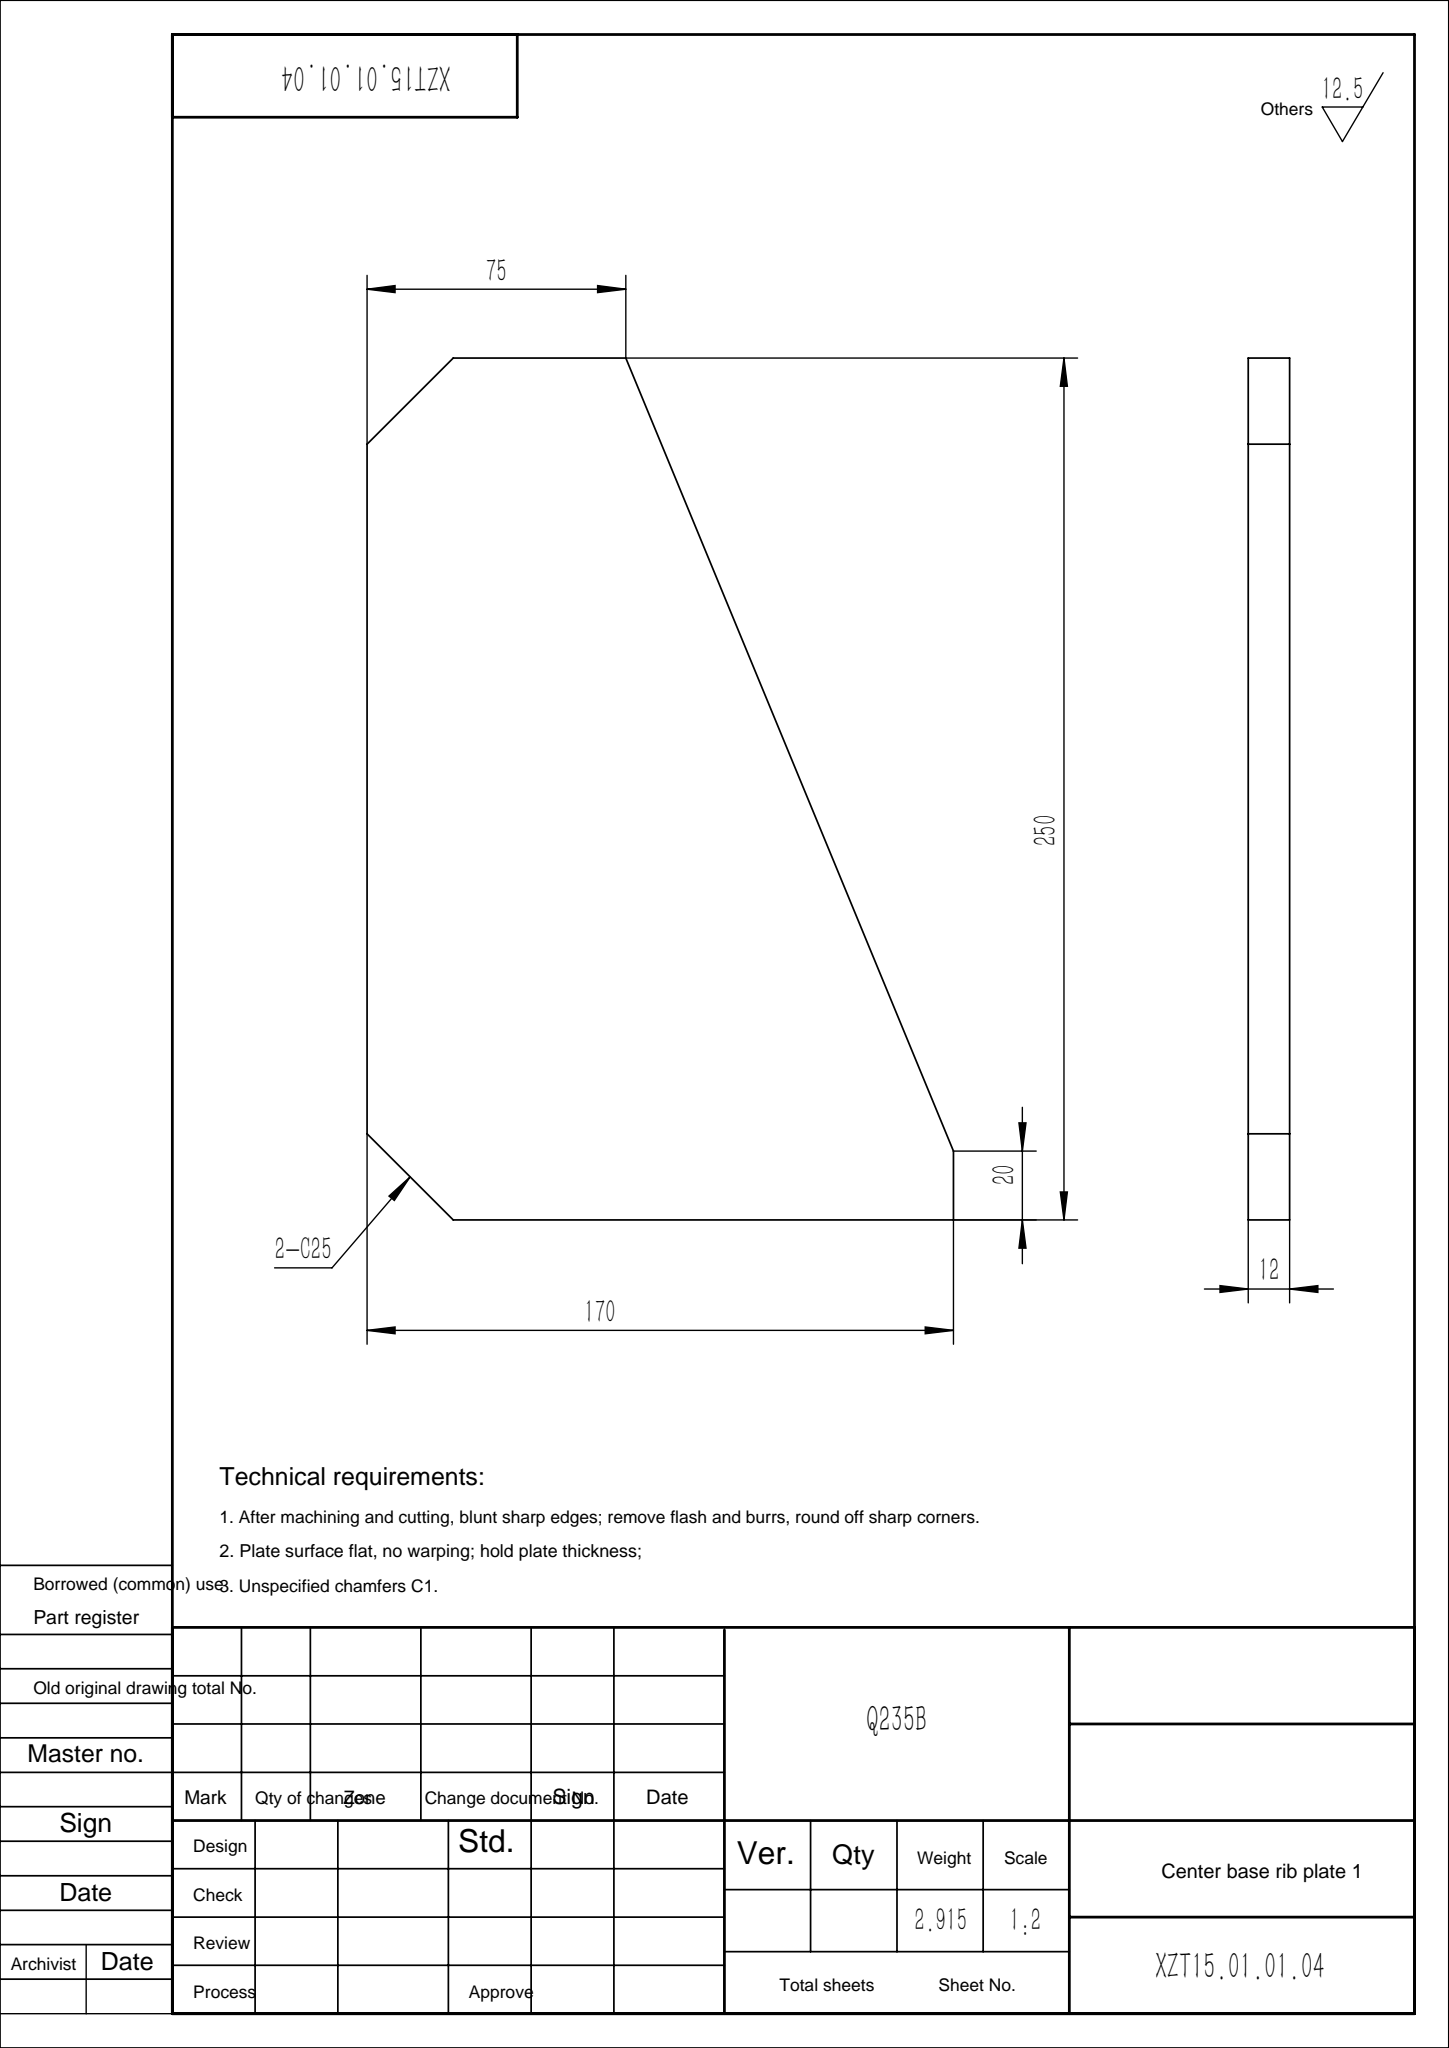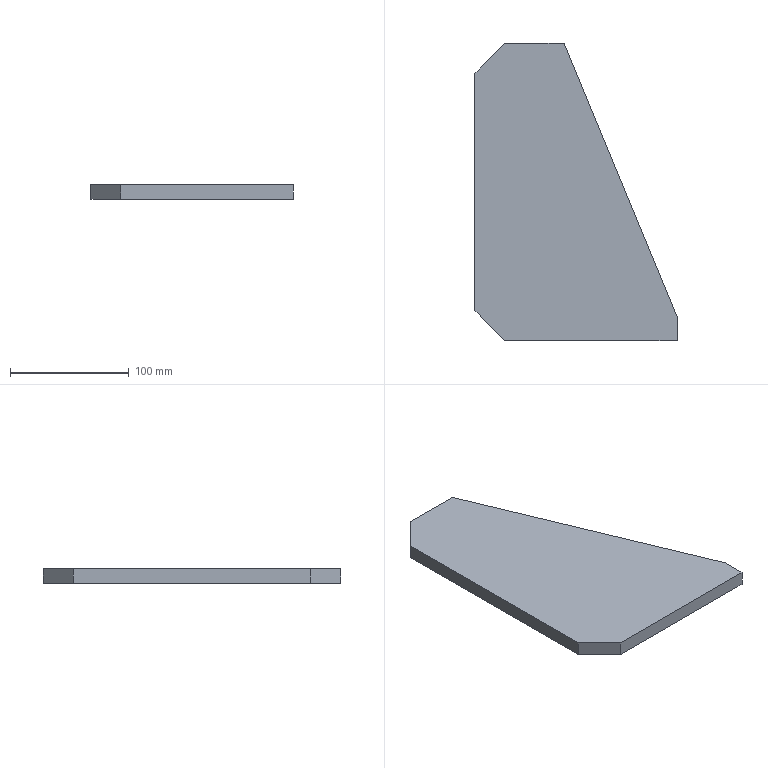Part | SolidWorks | features Chamfer 1, Extrusion 1 | 1 solid | 9 faces | box 170 x 250 x 12 mm | volume 371400 mm3 | plane 9
STEP:
#1=CARTESIAN_POINT('',(0.,225.,6.));
#2=VERTEX_POINT('',#1);
#3=CARTESIAN_POINT('',(0.,25.,6.));
#4=VERTEX_POINT('',#3);
#5=CARTESIAN_POINT('',(0.,250.,6.));
#6=DIRECTION('',(0.,-1.,0.));
#7=VECTOR('',#6,1000.);
#8=LINE('',#5,#7);
#9=EDGE_CURVE('',#2,#4,#8,.T.);
#10=ORIENTED_EDGE('',*,*,#9,.F.);
#11=CARTESIAN_POINT('',(0.,225.,-6.));
#12=VERTEX_POINT('',#11);
#13=CARTESIAN_POINT('',(0.,225.,6.));
#14=DIRECTION('',(0.,0.,-1.));
#15=VECTOR('',#14,1000.);
#16=LINE('',#13,#15);
#17=EDGE_CURVE('',#2,#12,#16,.T.);
#18=ORIENTED_EDGE('',*,*,#17,.T.);
#19=CARTESIAN_POINT('',(0.,25.,-6.));
#20=VERTEX_POINT('',#19);
#21=CARTESIAN_POINT('',(0.,250.,-6.));
#22=DIRECTION('',(0.,-1.,0.));
#23=VECTOR('',#22,1000.);
#24=LINE('',#21,#23);
#25=EDGE_CURVE('',#12,#20,#24,.T.);
#26=ORIENTED_EDGE('',*,*,#25,.T.);
#27=CARTESIAN_POINT('',(0.,25.,6.));
#28=DIRECTION('',(0.,0.,1.));
#29=VECTOR('',#28,1000.);
#30=LINE('',#27,#29);
#31=EDGE_CURVE('',#20,#4,#30,.T.);
#32=ORIENTED_EDGE('',*,*,#31,.T.);
#33=EDGE_LOOP('',(#10,#18,#26,#32));
#34=FACE_OUTER_BOUND('',#33,.T.);
#35=CARTESIAN_POINT('',(0.,250.,6.));
#36=DIRECTION('',(1.,0.,0.));
#37=DIRECTION('',(0.,1.,0.));
#38=AXIS2_PLACEMENT_3D('',#35,#36,#37);
#39=PLANE('',#38);
#40=ADVANCED_FACE('',(#34),#39,.F.);
#41=CARTESIAN_POINT('',(25.,0.,6.));
#42=VERTEX_POINT('',#41);
#43=CARTESIAN_POINT('',(170.,0.,6.));
#44=VERTEX_POINT('',#43);
#45=CARTESIAN_POINT('',(0.,0.,6.));
#46=DIRECTION('',(1.,0.,0.));
#47=VECTOR('',#46,1000.);
#48=LINE('',#45,#47);
#49=EDGE_CURVE('',#42,#44,#48,.T.);
#50=ORIENTED_EDGE('',*,*,#49,.F.);
#51=CARTESIAN_POINT('',(25.,0.,-6.));
#52=VERTEX_POINT('',#51);
#53=CARTESIAN_POINT('',(25.,0.,6.));
#54=DIRECTION('',(0.,0.,-1.));
#55=VECTOR('',#54,1000.);
#56=LINE('',#53,#55);
#57=EDGE_CURVE('',#42,#52,#56,.T.);
#58=ORIENTED_EDGE('',*,*,#57,.T.);
#59=CARTESIAN_POINT('',(170.,0.,-6.));
#60=VERTEX_POINT('',#59);
#61=CARTESIAN_POINT('',(0.,0.,-6.));
#62=DIRECTION('',(1.,0.,0.));
#63=VECTOR('',#62,1000.);
#64=LINE('',#61,#63);
#65=EDGE_CURVE('',#52,#60,#64,.T.);
#66=ORIENTED_EDGE('',*,*,#65,.T.);
#67=CARTESIAN_POINT('',(170.,0.,6.));
#68=DIRECTION('',(0.,0.,-1.));
#69=VECTOR('',#68,1000.);
#70=LINE('',#67,#69);
#71=EDGE_CURVE('',#44,#60,#70,.T.);
#72=ORIENTED_EDGE('',*,*,#71,.F.);
#73=EDGE_LOOP('',(#50,#58,#66,#72));
#74=FACE_OUTER_BOUND('',#73,.T.);
#75=CARTESIAN_POINT('',(0.,0.,6.));
#76=DIRECTION('',(0.,1.,0.));
#77=DIRECTION('',(0.,0.,1.));
#78=AXIS2_PLACEMENT_3D('',#75,#76,#77);
#79=PLANE('',#78);
#80=ADVANCED_FACE('',(#74),#79,.F.);
#81=CARTESIAN_POINT('',(170.,20.,-6.));
#82=VERTEX_POINT('',#81);
#83=CARTESIAN_POINT('',(170.,0.,-6.));
#84=DIRECTION('',(0.,1.,0.));
#85=VECTOR('',#84,1000.);
#86=LINE('',#83,#85);
#87=EDGE_CURVE('',#60,#82,#86,.T.);
#88=ORIENTED_EDGE('',*,*,#87,.T.);
#89=CARTESIAN_POINT('',(170.,20.,6.));
#90=VERTEX_POINT('',#89);
#91=CARTESIAN_POINT('',(170.,20.,6.));
#92=DIRECTION('',(0.,0.,-1.));
#93=VECTOR('',#92,1000.);
#94=LINE('',#91,#93);
#95=EDGE_CURVE('',#90,#82,#94,.T.);
#96=ORIENTED_EDGE('',*,*,#95,.F.);
#97=CARTESIAN_POINT('',(170.,0.,6.));
#98=DIRECTION('',(0.,1.,0.));
#99=VECTOR('',#98,1000.);
#100=LINE('',#97,#99);
#101=EDGE_CURVE('',#44,#90,#100,.T.);
#102=ORIENTED_EDGE('',*,*,#101,.F.);
#103=ORIENTED_EDGE('',*,*,#71,.T.);
#104=EDGE_LOOP('',(#88,#96,#102,#103));
#105=FACE_OUTER_BOUND('',#104,.T.);
#106=CARTESIAN_POINT('',(170.,0.,6.));
#107=DIRECTION('',(-1.,0.,0.));
#108=DIRECTION('',(0.,0.,1.));
#109=AXIS2_PLACEMENT_3D('',#106,#107,#108);
#110=PLANE('',#109);
#111=ADVANCED_FACE('',(#105),#110,.F.);
#112=CARTESIAN_POINT('',(75.,250.,-6.));
#113=VERTEX_POINT('',#112);
#114=CARTESIAN_POINT('',(170.,20.,-6.));
#115=DIRECTION('',(-0.3818,0.9243,0.));
#116=VECTOR('',#115,1000.);
#117=LINE('',#114,#116);
#118=EDGE_CURVE('',#82,#113,#117,.T.);
#119=ORIENTED_EDGE('',*,*,#118,.T.);
#120=CARTESIAN_POINT('',(75.,250.,6.));
#121=VERTEX_POINT('',#120);
#122=CARTESIAN_POINT('',(75.,250.,6.));
#123=DIRECTION('',(0.,0.,-1.));
#124=VECTOR('',#123,1000.);
#125=LINE('',#122,#124);
#126=EDGE_CURVE('',#121,#113,#125,.T.);
#127=ORIENTED_EDGE('',*,*,#126,.F.);
#128=CARTESIAN_POINT('',(170.,20.,6.));
#129=DIRECTION('',(-0.3818,0.9243,0.));
#130=VECTOR('',#129,1000.);
#131=LINE('',#128,#130);
#132=EDGE_CURVE('',#90,#121,#131,.T.);
#133=ORIENTED_EDGE('',*,*,#132,.F.);
#134=ORIENTED_EDGE('',*,*,#95,.T.);
#135=EDGE_LOOP('',(#119,#127,#133,#134));
#136=FACE_OUTER_BOUND('',#135,.T.);
#137=CARTESIAN_POINT('',(170.,20.,6.));
#138=DIRECTION('',(-0.9243,-0.3818,0.));
#139=DIRECTION('',(0.3818,-0.9243,0.));
#140=AXIS2_PLACEMENT_3D('',#137,#138,#139);
#141=PLANE('',#140);
#142=ADVANCED_FACE('',(#136),#141,.F.);
#143=CARTESIAN_POINT('',(25.,250.,-6.));
#144=VERTEX_POINT('',#143);
#145=CARTESIAN_POINT('',(75.,250.,-6.));
#146=DIRECTION('',(-1.,0.,0.));
#147=VECTOR('',#146,1000.);
#148=LINE('',#145,#147);
#149=EDGE_CURVE('',#113,#144,#148,.T.);
#150=ORIENTED_EDGE('',*,*,#149,.T.);
#151=CARTESIAN_POINT('',(25.,250.,6.));
#152=VERTEX_POINT('',#151);
#153=CARTESIAN_POINT('',(25.,250.,6.));
#154=DIRECTION('',(0.,0.,1.));
#155=VECTOR('',#154,1000.);
#156=LINE('',#153,#155);
#157=EDGE_CURVE('',#144,#152,#156,.T.);
#158=ORIENTED_EDGE('',*,*,#157,.T.);
#159=CARTESIAN_POINT('',(75.,250.,6.));
#160=DIRECTION('',(-1.,0.,0.));
#161=VECTOR('',#160,1000.);
#162=LINE('',#159,#161);
#163=EDGE_CURVE('',#121,#152,#162,.T.);
#164=ORIENTED_EDGE('',*,*,#163,.F.);
#165=ORIENTED_EDGE('',*,*,#126,.T.);
#166=EDGE_LOOP('',(#150,#158,#164,#165));
#167=FACE_OUTER_BOUND('',#166,.T.);
#168=CARTESIAN_POINT('',(75.,250.,6.));
#169=DIRECTION('',(0.,-1.,0.));
#170=DIRECTION('',(0.,0.,-1.));
#171=AXIS2_PLACEMENT_3D('',#168,#169,#170);
#172=PLANE('',#171);
#173=ADVANCED_FACE('',(#167),#172,.F.);
#174=ORIENTED_EDGE('',*,*,#163,.T.);
#175=CARTESIAN_POINT('',(-112.5,112.5,6.));
#176=DIRECTION('',(-0.7071,-0.7071,0.));
#177=VECTOR('',#176,1000.);
#178=LINE('',#175,#177);
#179=EDGE_CURVE('',#152,#2,#178,.T.);
#180=ORIENTED_EDGE('',*,*,#179,.T.);
#181=ORIENTED_EDGE('',*,*,#9,.T.);
#182=CARTESIAN_POINT('',(12.5,12.5,6.));
#183=DIRECTION('',(0.7071,-0.7071,0.));
#184=VECTOR('',#183,1000.);
#185=LINE('',#182,#184);
#186=EDGE_CURVE('',#4,#42,#185,.T.);
#187=ORIENTED_EDGE('',*,*,#186,.T.);
#188=ORIENTED_EDGE('',*,*,#49,.T.);
#189=ORIENTED_EDGE('',*,*,#101,.T.);
#190=ORIENTED_EDGE('',*,*,#132,.T.);
#191=EDGE_LOOP('',(#174,#180,#181,#187,#188,#189,#190));
#192=FACE_OUTER_BOUND('',#191,.T.);
#193=CARTESIAN_POINT('',(0.,0.,6.));
#194=DIRECTION('',(0.,0.,1.));
#195=DIRECTION('',(1.,0.,0.));
#196=AXIS2_PLACEMENT_3D('',#193,#194,#195);
#197=PLANE('',#196);
#198=ADVANCED_FACE('',(#192),#197,.T.);
#199=ORIENTED_EDGE('',*,*,#25,.F.);
#200=CARTESIAN_POINT('',(0.,225.,-6.));
#201=DIRECTION('',(0.7071,0.7071,0.));
#202=VECTOR('',#201,1000.);
#203=LINE('',#200,#202);
#204=EDGE_CURVE('',#12,#144,#203,.T.);
#205=ORIENTED_EDGE('',*,*,#204,.T.);
#206=ORIENTED_EDGE('',*,*,#149,.F.);
#207=ORIENTED_EDGE('',*,*,#118,.F.);
#208=ORIENTED_EDGE('',*,*,#87,.F.);
#209=ORIENTED_EDGE('',*,*,#65,.F.);
#210=CARTESIAN_POINT('',(25.,0.,-6.));
#211=DIRECTION('',(-0.7071,0.7071,0.));
#212=VECTOR('',#211,1000.);
#213=LINE('',#210,#212);
#214=EDGE_CURVE('',#52,#20,#213,.T.);
#215=ORIENTED_EDGE('',*,*,#214,.T.);
#216=EDGE_LOOP('',(#199,#205,#206,#207,#208,#209,#215));
#217=FACE_OUTER_BOUND('',#216,.T.);
#218=CARTESIAN_POINT('',(0.,0.,-6.));
#219=DIRECTION('',(0.,0.,1.));
#220=DIRECTION('',(1.,0.,0.));
#221=AXIS2_PLACEMENT_3D('',#218,#219,#220);
#222=PLANE('',#221);
#223=ADVANCED_FACE('',(#217),#222,.F.);
#224=ORIENTED_EDGE('',*,*,#179,.F.);
#225=ORIENTED_EDGE('',*,*,#157,.F.);
#226=ORIENTED_EDGE('',*,*,#204,.F.);
#227=ORIENTED_EDGE('',*,*,#17,.F.);
#228=EDGE_LOOP('',(#224,#225,#226,#227));
#229=FACE_OUTER_BOUND('',#228,.T.);
#230=CARTESIAN_POINT('',(0.,225.,6.));
#231=DIRECTION('',(0.7071,-0.7071,0.));
#232=DIRECTION('',(0.,0.,-1.));
#233=AXIS2_PLACEMENT_3D('',#230,#231,#232);
#234=PLANE('',#233);
#235=ADVANCED_FACE('',(#229),#234,.F.);
#236=ORIENTED_EDGE('',*,*,#186,.F.);
#237=ORIENTED_EDGE('',*,*,#31,.F.);
#238=ORIENTED_EDGE('',*,*,#214,.F.);
#239=ORIENTED_EDGE('',*,*,#57,.F.);
#240=EDGE_LOOP('',(#236,#237,#238,#239));
#241=FACE_OUTER_BOUND('',#240,.T.);
#242=CARTESIAN_POINT('',(25.,0.,6.));
#243=DIRECTION('',(0.7071,0.7071,0.));
#244=DIRECTION('',(0.,0.,-1.));
#245=AXIS2_PLACEMENT_3D('',#242,#243,#244);
#246=PLANE('',#245);
#247=ADVANCED_FACE('',(#241),#246,.F.);
#248=CLOSED_SHELL('',(#40,#80,#111,#142,#173,#198,#223,#235,#247));
#249=MANIFOLD_SOLID_BREP('',#248);
#250=CARTESIAN_POINT('',(0.,0.,0.));
#251=DIRECTION('',(0.,0.,1.));
#252=DIRECTION('',(1.,0.,0.));
#253=AXIS2_PLACEMENT_3D('',#250,#251,#252);
#254=(LENGTH_UNIT()NAMED_UNIT(*)SI_UNIT(.MILLI.,.METRE.));
#255=UNCERTAINTY_MEASURE_WITH_UNIT(LENGTH_MEASURE(0.00001),#254,'','');
#256=(NAMED_UNIT(*)PLANE_ANGLE_UNIT()SI_UNIT($,.RADIAN.));
#257=(NAMED_UNIT(*)SI_UNIT($,.STERADIAN.)SOLID_ANGLE_UNIT());
#258=(GEOMETRIC_REPRESENTATION_CONTEXT(3)GLOBAL_UNCERTAINTY_ASSIGNED_CONTEXT((#255))GLOBAL_UNIT_ASSIGNED_CONTEXT((#254,#256,#257))REPRESENTATION_CONTEXT('',''));
#259=ADVANCED_BREP_SHAPE_REPRESENTATION('',(#249,#253),#258);